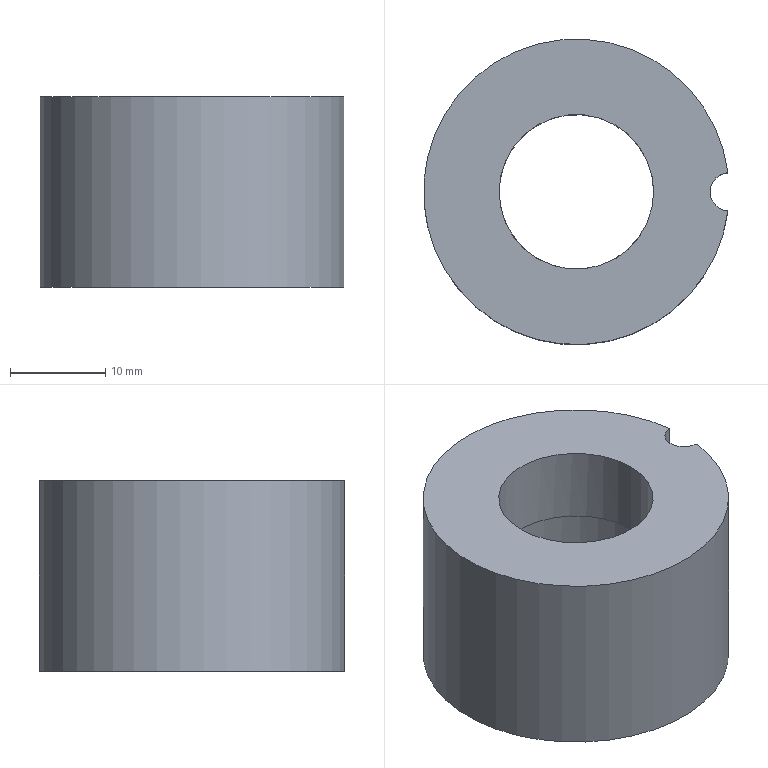Part | NX | features solid 2 | 1 solid | 7 faces | box 31.875 x 32 x 20 mm | volume 10316 mm3 | cylinder 4 | plane 3 | commonest cylinder face diameters 4 x1 16.19 x1 20.6 x1 32 x1
STEP:
#1=CARTESIAN_POINT('',(-368.125,22.004,115.008));
#2=VERTEX_POINT('',#1);
#3=CARTESIAN_POINT('',(-368.125,25.996,115.008));
#4=VERTEX_POINT('',#3);
#5=CARTESIAN_POINT('',(-368.,24.,115.008));
#6=DIRECTION('',(0.,0.,-1.));
#7=DIRECTION('',(-1.,0.,0.));
#8=AXIS2_PLACEMENT_3D('',#5,#6,#7);
#9=CIRCLE('',#8,2.);
#10=EDGE_CURVE('',#2,#4,#9,.T.);
#11=ORIENTED_EDGE('',*,*,#10,.T.);
#12=CARTESIAN_POINT('',(-384.,24.,115.008));
#13=DIRECTION('',(0.,0.,-1.));
#14=DIRECTION('',(-1.,0.,0.));
#15=AXIS2_PLACEMENT_3D('',#12,#13,#14);
#16=CIRCLE('',#15,16.);
#17=EDGE_CURVE('',#2,#4,#16,.T.);
#18=ORIENTED_EDGE('',*,*,#17,.F.);
#19=EDGE_LOOP('',(#11,#18));
#20=FACE_BOUND('',#19,.T.);
#21=CARTESIAN_POINT('',(-392.095,24.,115.008));
#22=VERTEX_POINT('',#21);
#23=CARTESIAN_POINT('',(-384.,24.,115.008));
#24=DIRECTION('',(0.,0.,-1.));
#25=DIRECTION('',(-1.,0.,0.));
#26=AXIS2_PLACEMENT_3D('',#23,#24,#25);
#27=CIRCLE('',#26,8.095);
#28=EDGE_CURVE('',#22,#22,#27,.T.);
#29=ORIENTED_EDGE('',*,*,#28,.T.);
#30=EDGE_LOOP('',(#29));
#31=FACE_BOUND('',#30,.T.);
#32=CARTESIAN_POINT('',(-384.,24.,115.008));
#33=DIRECTION('',(0.,0.,1.));
#34=DIRECTION('',(1.,0.,0.));
#35=AXIS2_PLACEMENT_3D('',#32,#33,#34);
#36=PLANE('',#35);
#37=ADVANCED_FACE('',(#20,#31),#36,.T.);
#38=CARTESIAN_POINT('',(-368.125,25.996,95.008));
#39=VERTEX_POINT('',#38);
#40=CARTESIAN_POINT('',(-368.125,22.004,95.008));
#41=VERTEX_POINT('',#40);
#42=CARTESIAN_POINT('',(-368.,24.,95.008));
#43=DIRECTION('',(0.,0.,1.));
#44=DIRECTION('',(1.,0.,0.));
#45=AXIS2_PLACEMENT_3D('',#42,#43,#44);
#46=CIRCLE('',#45,2.);
#47=EDGE_CURVE('',#39,#41,#46,.T.);
#48=ORIENTED_EDGE('',*,*,#47,.T.);
#49=CARTESIAN_POINT('',(-384.,24.,95.008));
#50=DIRECTION('',(0.,0.,1.));
#51=DIRECTION('',(1.,0.,0.));
#52=AXIS2_PLACEMENT_3D('',#49,#50,#51);
#53=CIRCLE('',#52,16.);
#54=EDGE_CURVE('',#39,#41,#53,.T.);
#55=ORIENTED_EDGE('',*,*,#54,.F.);
#56=EDGE_LOOP('',(#48,#55));
#57=FACE_BOUND('',#56,.T.);
#58=CARTESIAN_POINT('',(-373.7,24.,95.008));
#59=VERTEX_POINT('',#58);
#60=CARTESIAN_POINT('',(-384.,24.,95.008));
#61=DIRECTION('',(0.,0.,1.));
#62=DIRECTION('',(1.,0.,0.));
#63=AXIS2_PLACEMENT_3D('',#60,#61,#62);
#64=CIRCLE('',#63,10.3);
#65=EDGE_CURVE('',#59,#59,#64,.T.);
#66=ORIENTED_EDGE('',*,*,#65,.T.);
#67=EDGE_LOOP('',(#66));
#68=FACE_BOUND('',#67,.T.);
#69=CARTESIAN_POINT('',(-384.,24.,95.008));
#70=DIRECTION('',(0.,0.,-1.));
#71=DIRECTION('',(-1.,0.,0.));
#72=AXIS2_PLACEMENT_3D('',#69,#70,#71);
#73=PLANE('',#72);
#74=ADVANCED_FACE('',(#57,#68),#73,.T.);
#75=CARTESIAN_POINT('',(-368.125,25.996,105.008));
#76=DIRECTION('',(0.,0.,1.));
#77=VECTOR('',#76,1000.);
#78=LINE('',#75,#77);
#79=EDGE_CURVE('',#39,#4,#78,.T.);
#80=ORIENTED_EDGE('',*,*,#79,.F.);
#81=ORIENTED_EDGE('',*,*,#54,.T.);
#82=CARTESIAN_POINT('',(-368.125,22.004,105.008));
#83=DIRECTION('',(0.,0.,1.));
#84=VECTOR('',#83,1000.);
#85=LINE('',#82,#84);
#86=EDGE_CURVE('',#2,#41,#85,.F.);
#87=ORIENTED_EDGE('',*,*,#86,.F.);
#88=ORIENTED_EDGE('',*,*,#17,.T.);
#89=EDGE_LOOP('',(#80,#81,#87,#88));
#90=FACE_BOUND('',#89,.T.);
#91=CARTESIAN_POINT('',(-384.,24.,95.008));
#92=DIRECTION('',(0.,0.,1.));
#93=DIRECTION('',(1.,0.,0.));
#94=AXIS2_PLACEMENT_3D('',#91,#92,#93);
#95=CYLINDRICAL_SURFACE('',#94,16.);
#96=ADVANCED_FACE('',(#90),#95,.T.);
#97=CARTESIAN_POINT('',(-375.905,24.,107.008));
#98=VERTEX_POINT('',#97);
#99=CARTESIAN_POINT('',(-384.,24.,107.008));
#100=DIRECTION('',(0.,0.,1.));
#101=DIRECTION('',(1.,0.,0.));
#102=AXIS2_PLACEMENT_3D('',#99,#100,#101);
#103=CIRCLE('',#102,8.095);
#104=EDGE_CURVE('',#98,#98,#103,.T.);
#105=ORIENTED_EDGE('',*,*,#104,.T.);
#106=EDGE_LOOP('',(#105));
#107=FACE_BOUND('',#106,.T.);
#108=CARTESIAN_POINT('',(-394.3,24.,107.008));
#109=VERTEX_POINT('',#108);
#110=CARTESIAN_POINT('',(-384.,24.,107.008));
#111=DIRECTION('',(0.,0.,-1.));
#112=DIRECTION('',(-1.,0.,0.));
#113=AXIS2_PLACEMENT_3D('',#110,#111,#112);
#114=CIRCLE('',#113,10.3);
#115=EDGE_CURVE('',#109,#109,#114,.T.);
#116=ORIENTED_EDGE('',*,*,#115,.T.);
#117=EDGE_LOOP('',(#116));
#118=FACE_BOUND('',#117,.T.);
#119=CARTESIAN_POINT('',(-384.,24.,107.008));
#120=DIRECTION('',(0.,0.,1.));
#121=DIRECTION('',(1.,0.,0.));
#122=AXIS2_PLACEMENT_3D('',#119,#120,#121);
#123=PLANE('',#122);
#124=ADVANCED_FACE('',(#107,#118),#123,.F.);
#125=ORIENTED_EDGE('',*,*,#115,.F.);
#126=EDGE_LOOP('',(#125));
#127=FACE_BOUND('',#126,.T.);
#128=ORIENTED_EDGE('',*,*,#65,.F.);
#129=EDGE_LOOP('',(#128));
#130=FACE_BOUND('',#129,.T.);
#131=CARTESIAN_POINT('',(-384.,24.,95.008));
#132=DIRECTION('',(0.,0.,1.));
#133=DIRECTION('',(1.,0.,0.));
#134=AXIS2_PLACEMENT_3D('',#131,#132,#133);
#135=CYLINDRICAL_SURFACE('',#134,10.3);
#136=ADVANCED_FACE('',(#127,#130),#135,.F.);
#137=ORIENTED_EDGE('',*,*,#28,.F.);
#138=EDGE_LOOP('',(#137));
#139=FACE_BOUND('',#138,.T.);
#140=ORIENTED_EDGE('',*,*,#104,.F.);
#141=EDGE_LOOP('',(#140));
#142=FACE_BOUND('',#141,.T.);
#143=CARTESIAN_POINT('',(-384.,24.,107.008));
#144=DIRECTION('',(0.,0.,1.));
#145=DIRECTION('',(1.,0.,0.));
#146=AXIS2_PLACEMENT_3D('',#143,#144,#145);
#147=CYLINDRICAL_SURFACE('',#146,8.095);
#148=ADVANCED_FACE('',(#139,#142),#147,.F.);
#149=ORIENTED_EDGE('',*,*,#79,.T.);
#150=ORIENTED_EDGE('',*,*,#10,.F.);
#151=ORIENTED_EDGE('',*,*,#86,.T.);
#152=ORIENTED_EDGE('',*,*,#47,.F.);
#153=EDGE_LOOP('',(#149,#150,#151,#152));
#154=FACE_BOUND('',#153,.T.);
#155=CARTESIAN_POINT('',(-368.,24.,95.008));
#156=DIRECTION('',(0.,0.,1.));
#157=DIRECTION('',(1.,0.,0.));
#158=AXIS2_PLACEMENT_3D('',#155,#156,#157);
#159=CYLINDRICAL_SURFACE('',#158,2.);
#160=ADVANCED_FACE('',(#154),#159,.F.);
#161=CLOSED_SHELL('',(#37,#74,#96,#124,#136,#148,#160));
#162=MANIFOLD_SOLID_BREP('',#161);
#163=(LENGTH_UNIT()NAMED_UNIT(*)SI_UNIT(.MILLI.,.METRE.));
#164=UNCERTAINTY_MEASURE_WITH_UNIT(LENGTH_MEASURE(0.00001),#163,'','');
#165=(NAMED_UNIT(*)PLANE_ANGLE_UNIT()SI_UNIT($,.RADIAN.));
#166=(NAMED_UNIT(*)SI_UNIT($,.STERADIAN.)SOLID_ANGLE_UNIT());
#167=(GEOMETRIC_REPRESENTATION_CONTEXT(3)GLOBAL_UNCERTAINTY_ASSIGNED_CONTEXT((#164))GLOBAL_UNIT_ASSIGNED_CONTEXT((#163,#165,#166))REPRESENTATION_CONTEXT('',''));
#168=ADVANCED_BREP_SHAPE_REPRESENTATION('',(#162),#167);